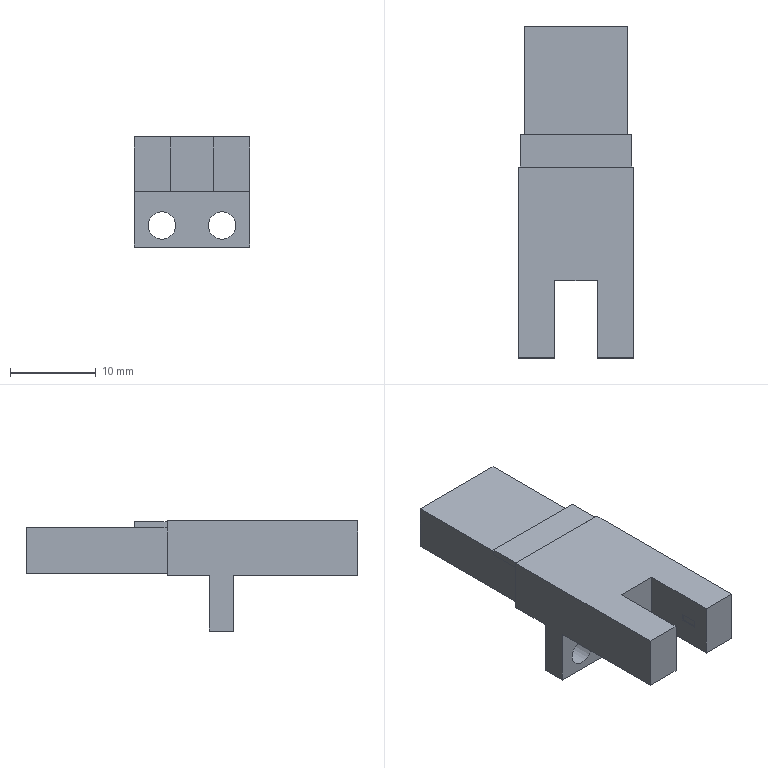Part | NX | 1 solid | 269 faces | box 13.4 x 38.6 x 12.8 mm | volume 2876 mm3 | plane 263 | cylinder 6 | commonest cylinder face diameters 3.2 x4 1.6 x2